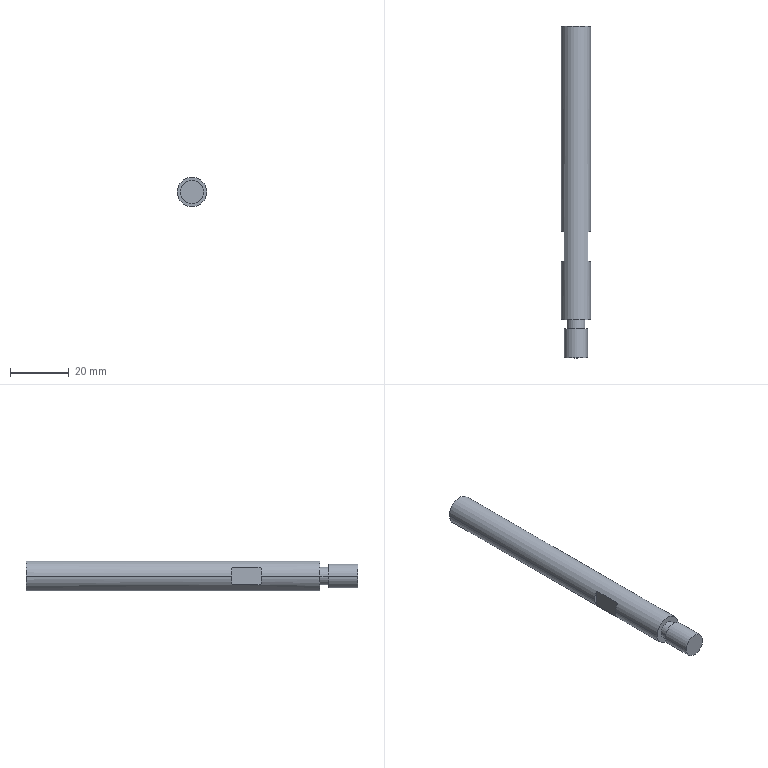Part | SolidWorks | features HoleWzd 1, ICE 1, Revolution 1 | 1 solid | 20 faces | box 10 x 113 x 10 mm | volume 8114 mm3 | plane 10 | cylinder 8 | cone 2 | commonest cylinder face diameters 5 x2 6 x2 8 x2 10 x2
STEP:
#1=CARTESIAN_POINT('',(0.,2.171,-2.5));
#2=VERTEX_POINT('',#1);
#3=CARTESIAN_POINT('',(0.,2.171,2.5));
#4=VERTEX_POINT('',#3);
#5=CARTESIAN_POINT('',(0.,2.171,0.));
#6=DIRECTION('',(0.,1.,0.));
#7=DIRECTION('',(0.,0.,1.));
#8=AXIS2_PLACEMENT_3D('',#5,#6,#7);
#9=CIRCLE('',#8,2.5);
#10=EDGE_CURVE('',#2,#4,#9,.T.);
#11=ORIENTED_EDGE('',*,*,#10,.F.);
#12=CARTESIAN_POINT('',(0.,14.171,-2.5));
#13=VERTEX_POINT('',#12);
#14=CARTESIAN_POINT('',(0.,14.171,-2.5));
#15=DIRECTION('',(0.,1.,0.));
#16=VECTOR('',#15,1000.);
#17=LINE('',#14,#16);
#18=EDGE_CURVE('',#2,#13,#17,.T.);
#19=ORIENTED_EDGE('',*,*,#18,.T.);
#20=CARTESIAN_POINT('',(0.,14.171,2.5));
#21=VERTEX_POINT('',#20);
#22=CARTESIAN_POINT('',(0.,14.171,0.));
#23=DIRECTION('',(0.,1.,0.));
#24=DIRECTION('',(0.,0.,1.));
#25=AXIS2_PLACEMENT_3D('',#22,#23,#24);
#26=CIRCLE('',#25,2.5);
#27=EDGE_CURVE('',#13,#21,#26,.T.);
#28=ORIENTED_EDGE('',*,*,#27,.T.);
#29=CARTESIAN_POINT('',(0.,14.171,2.5));
#30=DIRECTION('',(0.,1.,0.));
#31=VECTOR('',#30,1000.);
#32=LINE('',#29,#31);
#33=EDGE_CURVE('',#4,#21,#32,.T.);
#34=ORIENTED_EDGE('',*,*,#33,.F.);
#35=EDGE_LOOP('',(#11,#19,#28,#34));
#36=FACE_OUTER_BOUND('',#35,.T.);
#37=CARTESIAN_POINT('',(0.,14.171,0.));
#38=DIRECTION('',(0.,1.,0.));
#39=DIRECTION('',(0.,0.,1.));
#40=AXIS2_PLACEMENT_3D('',#37,#38,#39);
#41=CYLINDRICAL_SURFACE('',#40,2.5);
#42=ADVANCED_FACE('',(#36),#41,.F.);
#43=CARTESIAN_POINT('',(0.,0.6688,0.));
#44=VERTEX_POINT('',#43);
#45=CARTESIAN_POINT('',(0.,2.171,2.5));
#46=DIRECTION('',(0.,0.515,0.8572));
#47=VECTOR('',#46,1000.);
#48=LINE('',#45,#47);
#49=EDGE_CURVE('',#44,#4,#48,.T.);
#50=ORIENTED_EDGE('',*,*,#49,.F.);
#51=CARTESIAN_POINT('',(0.,2.171,-2.5));
#52=DIRECTION('',(0.,0.515,-0.8572));
#53=VECTOR('',#52,1000.);
#54=LINE('',#51,#53);
#55=EDGE_CURVE('',#44,#2,#54,.T.);
#56=ORIENTED_EDGE('',*,*,#55,.T.);
#57=ORIENTED_EDGE('',*,*,#10,.T.);
#58=EDGE_LOOP('',(#50,#56,#57));
#59=FACE_OUTER_BOUND('',#58,.T.);
#60=CARTESIAN_POINT('',(0.,2.171,0.));
#61=DIRECTION('',(0.,1.,0.));
#62=DIRECTION('',(0.,0.,1.));
#63=AXIS2_PLACEMENT_3D('',#60,#61,#62);
#64=CONICAL_SURFACE('',#63,2.5,1.03);
#65=ADVANCED_FACE('',(#59),#64,.F.);
#66=CARTESIAN_POINT('',(-5.,-85.829,0.));
#67=VERTEX_POINT('',#66);
#68=CARTESIAN_POINT('',(5.,-85.829,0.));
#69=VERTEX_POINT('',#68);
#70=CARTESIAN_POINT('',(0.,-85.829,0.));
#71=DIRECTION('',(0.,1.,0.));
#72=DIRECTION('',(-1.,0.,0.));
#73=AXIS2_PLACEMENT_3D('',#70,#71,#72);
#74=CIRCLE('',#73,5.);
#75=EDGE_CURVE('',#67,#69,#74,.T.);
#76=ORIENTED_EDGE('',*,*,#75,.T.);
#77=CARTESIAN_POINT('',(5.,-65.829,0.));
#78=VERTEX_POINT('',#77);
#79=CARTESIAN_POINT('',(5.,14.171,0.));
#80=DIRECTION('',(0.,1.,0.));
#81=VECTOR('',#80,1000.);
#82=LINE('',#79,#81);
#83=EDGE_CURVE('',#69,#78,#82,.T.);
#84=ORIENTED_EDGE('',*,*,#83,.T.);
#85=CARTESIAN_POINT('',(4.,-65.829,3.));
#86=VERTEX_POINT('',#85);
#87=CARTESIAN_POINT('',(0.,-65.829,0.));
#88=DIRECTION('',(0.,1.,0.));
#89=DIRECTION('',(0.,0.,-1.));
#90=AXIS2_PLACEMENT_3D('',#87,#88,#89);
#91=CIRCLE('',#90,5.);
#92=EDGE_CURVE('',#86,#78,#91,.T.);
#93=ORIENTED_EDGE('',*,*,#92,.F.);
#94=CARTESIAN_POINT('',(4.,-55.829,3.));
#95=VERTEX_POINT('',#94);
#96=CARTESIAN_POINT('',(4.,14.171,3.));
#97=DIRECTION('',(0.,-1.,0.));
#98=VECTOR('',#97,1000.);
#99=LINE('',#96,#98);
#100=EDGE_CURVE('',#95,#86,#99,.T.);
#101=ORIENTED_EDGE('',*,*,#100,.F.);
#102=CARTESIAN_POINT('',(5.,-55.829,0.));
#103=VERTEX_POINT('',#102);
#104=CARTESIAN_POINT('',(0.,-55.829,0.));
#105=DIRECTION('',(0.,-1.,0.));
#106=DIRECTION('',(0.,0.,1.));
#107=AXIS2_PLACEMENT_3D('',#104,#105,#106);
#108=CIRCLE('',#107,5.);
#109=EDGE_CURVE('',#103,#95,#108,.T.);
#110=ORIENTED_EDGE('',*,*,#109,.F.);
#111=CARTESIAN_POINT('',(5.,14.171,0.));
#112=VERTEX_POINT('',#111);
#113=CARTESIAN_POINT('',(5.,14.171,0.));
#114=DIRECTION('',(0.,1.,0.));
#115=VECTOR('',#114,1000.);
#116=LINE('',#113,#115);
#117=EDGE_CURVE('',#103,#112,#116,.T.);
#118=ORIENTED_EDGE('',*,*,#117,.T.);
#119=CARTESIAN_POINT('',(-5.,14.171,0.));
#120=VERTEX_POINT('',#119);
#121=CARTESIAN_POINT('',(0.,14.171,0.));
#122=DIRECTION('',(0.,1.,0.));
#123=DIRECTION('',(-1.,0.,0.));
#124=AXIS2_PLACEMENT_3D('',#121,#122,#123);
#125=CIRCLE('',#124,5.);
#126=EDGE_CURVE('',#120,#112,#125,.T.);
#127=ORIENTED_EDGE('',*,*,#126,.F.);
#128=CARTESIAN_POINT('',(-5.,-55.829,0.));
#129=VERTEX_POINT('',#128);
#130=CARTESIAN_POINT('',(-5.,14.171,0.));
#131=DIRECTION('',(0.,1.,0.));
#132=VECTOR('',#131,1000.);
#133=LINE('',#130,#132);
#134=EDGE_CURVE('',#129,#120,#133,.T.);
#135=ORIENTED_EDGE('',*,*,#134,.F.);
#136=CARTESIAN_POINT('',(-4.,-55.829,3.));
#137=VERTEX_POINT('',#136);
#138=CARTESIAN_POINT('',(0.,-55.829,0.));
#139=DIRECTION('',(0.,-1.,0.));
#140=DIRECTION('',(0.,0.,1.));
#141=AXIS2_PLACEMENT_3D('',#138,#139,#140);
#142=CIRCLE('',#141,5.);
#143=EDGE_CURVE('',#137,#129,#142,.T.);
#144=ORIENTED_EDGE('',*,*,#143,.F.);
#145=CARTESIAN_POINT('',(-4.,-65.829,3.));
#146=VERTEX_POINT('',#145);
#147=CARTESIAN_POINT('',(-4.,14.171,3.));
#148=DIRECTION('',(0.,1.,0.));
#149=VECTOR('',#148,1000.);
#150=LINE('',#147,#149);
#151=EDGE_CURVE('',#146,#137,#150,.T.);
#152=ORIENTED_EDGE('',*,*,#151,.F.);
#153=CARTESIAN_POINT('',(-5.,-65.829,0.));
#154=VERTEX_POINT('',#153);
#155=CARTESIAN_POINT('',(0.,-65.829,0.));
#156=DIRECTION('',(0.,1.,0.));
#157=DIRECTION('',(0.,0.,-1.));
#158=AXIS2_PLACEMENT_3D('',#155,#156,#157);
#159=CIRCLE('',#158,5.);
#160=EDGE_CURVE('',#154,#146,#159,.T.);
#161=ORIENTED_EDGE('',*,*,#160,.F.);
#162=CARTESIAN_POINT('',(-5.,14.171,0.));
#163=DIRECTION('',(0.,1.,0.));
#164=VECTOR('',#163,1000.);
#165=LINE('',#162,#164);
#166=EDGE_CURVE('',#67,#154,#165,.T.);
#167=ORIENTED_EDGE('',*,*,#166,.F.);
#168=EDGE_LOOP('',(#76,#84,#93,#101,#110,#118,#127,#135,#144,#152,#161,#167));
#169=FACE_OUTER_BOUND('',#168,.T.);
#170=CARTESIAN_POINT('',(0.,14.171,0.));
#171=DIRECTION('',(0.,1.,0.));
#172=DIRECTION('',(-1.,0.,0.));
#173=AXIS2_PLACEMENT_3D('',#170,#171,#172);
#174=CYLINDRICAL_SURFACE('',#173,5.);
#175=ADVANCED_FACE('',(#169),#174,.T.);
#176=CARTESIAN_POINT('',(-3.,-88.829,0.));
#177=VERTEX_POINT('',#176);
#178=CARTESIAN_POINT('',(3.,-88.829,0.));
#179=VERTEX_POINT('',#178);
#180=CARTESIAN_POINT('',(0.,-88.829,0.));
#181=DIRECTION('',(0.,1.,0.));
#182=DIRECTION('',(-1.,0.,0.));
#183=AXIS2_PLACEMENT_3D('',#180,#181,#182);
#184=CIRCLE('',#183,3.);
#185=EDGE_CURVE('',#177,#179,#184,.T.);
#186=ORIENTED_EDGE('',*,*,#185,.T.);
#187=CARTESIAN_POINT('',(3.,-85.829,0.));
#188=VERTEX_POINT('',#187);
#189=CARTESIAN_POINT('',(3.,14.171,0.));
#190=DIRECTION('',(0.,1.,0.));
#191=VECTOR('',#190,1000.);
#192=LINE('',#189,#191);
#193=EDGE_CURVE('',#179,#188,#192,.T.);
#194=ORIENTED_EDGE('',*,*,#193,.T.);
#195=CARTESIAN_POINT('',(-3.,-85.829,0.));
#196=VERTEX_POINT('',#195);
#197=CARTESIAN_POINT('',(0.,-85.829,0.));
#198=DIRECTION('',(0.,1.,0.));
#199=DIRECTION('',(-1.,0.,0.));
#200=AXIS2_PLACEMENT_3D('',#197,#198,#199);
#201=CIRCLE('',#200,3.);
#202=EDGE_CURVE('',#196,#188,#201,.T.);
#203=ORIENTED_EDGE('',*,*,#202,.F.);
#204=CARTESIAN_POINT('',(-3.,14.171,0.));
#205=DIRECTION('',(0.,1.,0.));
#206=VECTOR('',#205,1000.);
#207=LINE('',#204,#206);
#208=EDGE_CURVE('',#177,#196,#207,.T.);
#209=ORIENTED_EDGE('',*,*,#208,.F.);
#210=EDGE_LOOP('',(#186,#194,#203,#209));
#211=FACE_OUTER_BOUND('',#210,.T.);
#212=CARTESIAN_POINT('',(0.,14.171,0.));
#213=DIRECTION('',(0.,1.,0.));
#214=DIRECTION('',(-1.,0.,0.));
#215=AXIS2_PLACEMENT_3D('',#212,#213,#214);
#216=CYLINDRICAL_SURFACE('',#215,3.);
#217=ADVANCED_FACE('',(#211),#216,.T.);
#218=CARTESIAN_POINT('',(-4.,-98.829,0.));
#219=VERTEX_POINT('',#218);
#220=CARTESIAN_POINT('',(4.,-98.829,0.));
#221=VERTEX_POINT('',#220);
#222=CARTESIAN_POINT('',(0.,-98.829,0.));
#223=DIRECTION('',(0.,1.,0.));
#224=DIRECTION('',(-1.,0.,0.));
#225=AXIS2_PLACEMENT_3D('',#222,#223,#224);
#226=CIRCLE('',#225,4.);
#227=EDGE_CURVE('',#219,#221,#226,.T.);
#228=ORIENTED_EDGE('',*,*,#227,.T.);
#229=CARTESIAN_POINT('',(4.,-88.829,0.));
#230=VERTEX_POINT('',#229);
#231=CARTESIAN_POINT('',(4.,14.171,0.));
#232=DIRECTION('',(0.,1.,0.));
#233=VECTOR('',#232,1000.);
#234=LINE('',#231,#233);
#235=EDGE_CURVE('',#221,#230,#234,.T.);
#236=ORIENTED_EDGE('',*,*,#235,.T.);
#237=CARTESIAN_POINT('',(-4.,-88.829,0.));
#238=VERTEX_POINT('',#237);
#239=CARTESIAN_POINT('',(0.,-88.829,0.));
#240=DIRECTION('',(0.,1.,0.));
#241=DIRECTION('',(-1.,0.,0.));
#242=AXIS2_PLACEMENT_3D('',#239,#240,#241);
#243=CIRCLE('',#242,4.);
#244=EDGE_CURVE('',#238,#230,#243,.T.);
#245=ORIENTED_EDGE('',*,*,#244,.F.);
#246=CARTESIAN_POINT('',(-4.,14.171,0.));
#247=DIRECTION('',(0.,1.,0.));
#248=VECTOR('',#247,1000.);
#249=LINE('',#246,#248);
#250=EDGE_CURVE('',#219,#238,#249,.T.);
#251=ORIENTED_EDGE('',*,*,#250,.F.);
#252=EDGE_LOOP('',(#228,#236,#245,#251));
#253=FACE_OUTER_BOUND('',#252,.T.);
#254=CARTESIAN_POINT('',(0.,14.171,0.));
#255=DIRECTION('',(0.,1.,0.));
#256=DIRECTION('',(-1.,0.,0.));
#257=AXIS2_PLACEMENT_3D('',#254,#255,#256);
#258=CYLINDRICAL_SURFACE('',#257,4.);
#259=ADVANCED_FACE('',(#253),#258,.T.);
#260=CARTESIAN_POINT('',(0.,14.171,0.));
#261=DIRECTION('',(0.,1.,0.));
#262=DIRECTION('',(0.,0.,1.));
#263=AXIS2_PLACEMENT_3D('',#260,#261,#262);
#264=CIRCLE('',#263,2.5);
#265=EDGE_CURVE('',#21,#13,#264,.T.);
#266=ORIENTED_EDGE('',*,*,#265,.F.);
#267=ORIENTED_EDGE('',*,*,#27,.F.);
#268=EDGE_LOOP('',(#266,#267));
#269=FACE_BOUND('',#268,.T.);
#270=ORIENTED_EDGE('',*,*,#126,.T.);
#271=CARTESIAN_POINT('',(0.,14.171,0.));
#272=DIRECTION('',(0.,1.,0.));
#273=DIRECTION('',(-1.,0.,0.));
#274=AXIS2_PLACEMENT_3D('',#271,#272,#273);
#275=CIRCLE('',#274,5.);
#276=EDGE_CURVE('',#112,#120,#275,.T.);
#277=ORIENTED_EDGE('',*,*,#276,.T.);
#278=EDGE_LOOP('',(#270,#277));
#279=FACE_OUTER_BOUND('',#278,.T.);
#280=CARTESIAN_POINT('',(-5.,14.171,0.));
#281=DIRECTION('',(0.,1.,0.));
#282=DIRECTION('',(-1.,0.,0.));
#283=AXIS2_PLACEMENT_3D('',#280,#281,#282);
#284=PLANE('',#283);
#285=ADVANCED_FACE('',(#269,#279),#284,.T.);
#286=ORIENTED_EDGE('',*,*,#227,.F.);
#287=CARTESIAN_POINT('',(0.,-98.829,0.));
#288=DIRECTION('',(0.,1.,0.));
#289=DIRECTION('',(-1.,0.,0.));
#290=AXIS2_PLACEMENT_3D('',#287,#288,#289);
#291=CIRCLE('',#290,4.);
#292=EDGE_CURVE('',#221,#219,#291,.T.);
#293=ORIENTED_EDGE('',*,*,#292,.F.);
#294=EDGE_LOOP('',(#286,#293));
#295=FACE_OUTER_BOUND('',#294,.T.);
#296=CARTESIAN_POINT('',(0.,-98.829,0.));
#297=DIRECTION('',(0.,-1.,0.));
#298=DIRECTION('',(1.,0.,0.));
#299=AXIS2_PLACEMENT_3D('',#296,#297,#298);
#300=PLANE('',#299);
#301=ADVANCED_FACE('',(#295),#300,.T.);
#302=ORIENTED_EDGE('',*,*,#235,.F.);
#303=ORIENTED_EDGE('',*,*,#292,.T.);
#304=ORIENTED_EDGE('',*,*,#250,.T.);
#305=CARTESIAN_POINT('',(0.,-88.829,0.));
#306=DIRECTION('',(0.,1.,0.));
#307=DIRECTION('',(-1.,0.,0.));
#308=AXIS2_PLACEMENT_3D('',#305,#306,#307);
#309=CIRCLE('',#308,4.);
#310=EDGE_CURVE('',#230,#238,#309,.T.);
#311=ORIENTED_EDGE('',*,*,#310,.F.);
#312=EDGE_LOOP('',(#302,#303,#304,#311));
#313=FACE_OUTER_BOUND('',#312,.T.);
#314=CARTESIAN_POINT('',(0.,14.171,0.));
#315=DIRECTION('',(0.,1.,0.));
#316=DIRECTION('',(-1.,0.,0.));
#317=AXIS2_PLACEMENT_3D('',#314,#315,#316);
#318=CYLINDRICAL_SURFACE('',#317,4.);
#319=ADVANCED_FACE('',(#313),#318,.T.);
#320=ORIENTED_EDGE('',*,*,#244,.T.);
#321=ORIENTED_EDGE('',*,*,#310,.T.);
#322=EDGE_LOOP('',(#320,#321));
#323=FACE_OUTER_BOUND('',#322,.T.);
#324=ORIENTED_EDGE('',*,*,#185,.F.);
#325=CARTESIAN_POINT('',(0.,-88.829,0.));
#326=DIRECTION('',(0.,1.,0.));
#327=DIRECTION('',(-1.,0.,0.));
#328=AXIS2_PLACEMENT_3D('',#325,#326,#327);
#329=CIRCLE('',#328,3.);
#330=EDGE_CURVE('',#179,#177,#329,.T.);
#331=ORIENTED_EDGE('',*,*,#330,.F.);
#332=EDGE_LOOP('',(#324,#331));
#333=FACE_BOUND('',#332,.T.);
#334=CARTESIAN_POINT('',(-4.,-88.829,0.));
#335=DIRECTION('',(0.,1.,0.));
#336=DIRECTION('',(-1.,0.,0.));
#337=AXIS2_PLACEMENT_3D('',#334,#335,#336);
#338=PLANE('',#337);
#339=ADVANCED_FACE('',(#323,#333),#338,.T.);
#340=ORIENTED_EDGE('',*,*,#193,.F.);
#341=ORIENTED_EDGE('',*,*,#330,.T.);
#342=ORIENTED_EDGE('',*,*,#208,.T.);
#343=CARTESIAN_POINT('',(0.,-85.829,0.));
#344=DIRECTION('',(0.,1.,0.));
#345=DIRECTION('',(-1.,0.,0.));
#346=AXIS2_PLACEMENT_3D('',#343,#344,#345);
#347=CIRCLE('',#346,3.);
#348=EDGE_CURVE('',#188,#196,#347,.T.);
#349=ORIENTED_EDGE('',*,*,#348,.F.);
#350=EDGE_LOOP('',(#340,#341,#342,#349));
#351=FACE_OUTER_BOUND('',#350,.T.);
#352=CARTESIAN_POINT('',(0.,14.171,0.));
#353=DIRECTION('',(0.,1.,0.));
#354=DIRECTION('',(-1.,0.,0.));
#355=AXIS2_PLACEMENT_3D('',#352,#353,#354);
#356=CYLINDRICAL_SURFACE('',#355,3.);
#357=ADVANCED_FACE('',(#351),#356,.T.);
#358=ORIENTED_EDGE('',*,*,#202,.T.);
#359=ORIENTED_EDGE('',*,*,#348,.T.);
#360=EDGE_LOOP('',(#358,#359));
#361=FACE_BOUND('',#360,.T.);
#362=ORIENTED_EDGE('',*,*,#75,.F.);
#363=CARTESIAN_POINT('',(0.,-85.829,0.));
#364=DIRECTION('',(0.,1.,0.));
#365=DIRECTION('',(-1.,0.,0.));
#366=AXIS2_PLACEMENT_3D('',#363,#364,#365);
#367=CIRCLE('',#366,5.);
#368=EDGE_CURVE('',#69,#67,#367,.T.);
#369=ORIENTED_EDGE('',*,*,#368,.F.);
#370=EDGE_LOOP('',(#362,#369));
#371=FACE_OUTER_BOUND('',#370,.T.);
#372=CARTESIAN_POINT('',(-3.,-85.829,0.));
#373=DIRECTION('',(0.,-1.,0.));
#374=DIRECTION('',(1.,0.,0.));
#375=AXIS2_PLACEMENT_3D('',#372,#373,#374);
#376=PLANE('',#375);
#377=ADVANCED_FACE('',(#361,#371),#376,.T.);
#378=ORIENTED_EDGE('',*,*,#83,.F.);
#379=ORIENTED_EDGE('',*,*,#368,.T.);
#380=ORIENTED_EDGE('',*,*,#166,.T.);
#381=CARTESIAN_POINT('',(-4.,-65.829,-3.));
#382=VERTEX_POINT('',#381);
#383=CARTESIAN_POINT('',(0.,-65.829,0.));
#384=DIRECTION('',(0.,1.,0.));
#385=DIRECTION('',(0.,0.,-1.));
#386=AXIS2_PLACEMENT_3D('',#383,#384,#385);
#387=CIRCLE('',#386,5.);
#388=EDGE_CURVE('',#382,#154,#387,.T.);
#389=ORIENTED_EDGE('',*,*,#388,.F.);
#390=CARTESIAN_POINT('',(-4.,-55.829,-3.));
#391=VERTEX_POINT('',#390);
#392=CARTESIAN_POINT('',(-4.,14.171,-3.));
#393=DIRECTION('',(0.,-1.,0.));
#394=VECTOR('',#393,1000.);
#395=LINE('',#392,#394);
#396=EDGE_CURVE('',#391,#382,#395,.T.);
#397=ORIENTED_EDGE('',*,*,#396,.F.);
#398=CARTESIAN_POINT('',(0.,-55.829,0.));
#399=DIRECTION('',(0.,-1.,0.));
#400=DIRECTION('',(0.,0.,1.));
#401=AXIS2_PLACEMENT_3D('',#398,#399,#400);
#402=CIRCLE('',#401,5.);
#403=EDGE_CURVE('',#129,#391,#402,.T.);
#404=ORIENTED_EDGE('',*,*,#403,.F.);
#405=ORIENTED_EDGE('',*,*,#134,.T.);
#406=ORIENTED_EDGE('',*,*,#276,.F.);
#407=ORIENTED_EDGE('',*,*,#117,.F.);
#408=CARTESIAN_POINT('',(4.,-55.829,-3.));
#409=VERTEX_POINT('',#408);
#410=CARTESIAN_POINT('',(0.,-55.829,0.));
#411=DIRECTION('',(0.,-1.,0.));
#412=DIRECTION('',(0.,0.,1.));
#413=AXIS2_PLACEMENT_3D('',#410,#411,#412);
#414=CIRCLE('',#413,5.);
#415=EDGE_CURVE('',#409,#103,#414,.T.);
#416=ORIENTED_EDGE('',*,*,#415,.F.);
#417=CARTESIAN_POINT('',(4.,-65.829,-3.));
#418=VERTEX_POINT('',#417);
#419=CARTESIAN_POINT('',(4.,14.171,-3.));
#420=DIRECTION('',(0.,1.,0.));
#421=VECTOR('',#420,1000.);
#422=LINE('',#419,#421);
#423=EDGE_CURVE('',#418,#409,#422,.T.);
#424=ORIENTED_EDGE('',*,*,#423,.F.);
#425=CARTESIAN_POINT('',(0.,-65.829,0.));
#426=DIRECTION('',(0.,1.,0.));
#427=DIRECTION('',(0.,0.,-1.));
#428=AXIS2_PLACEMENT_3D('',#425,#426,#427);
#429=CIRCLE('',#428,5.);
#430=EDGE_CURVE('',#78,#418,#429,.T.);
#431=ORIENTED_EDGE('',*,*,#430,.F.);
#432=EDGE_LOOP('',(#378,#379,#380,#389,#397,#404,#405,#406,#407,#416,#424,#431));
#433=FACE_OUTER_BOUND('',#432,.T.);
#434=CARTESIAN_POINT('',(0.,14.171,0.));
#435=DIRECTION('',(0.,1.,0.));
#436=DIRECTION('',(-1.,0.,0.));
#437=AXIS2_PLACEMENT_3D('',#434,#435,#436);
#438=CYLINDRICAL_SURFACE('',#437,5.);
#439=ADVANCED_FACE('',(#433),#438,.T.);
#440=ORIENTED_EDGE('',*,*,#415,.T.);
#441=ORIENTED_EDGE('',*,*,#109,.T.);
#442=CARTESIAN_POINT('',(4.,-55.829,-5.));
#443=DIRECTION('',(0.,0.,1.));
#444=VECTOR('',#443,1000.);
#445=LINE('',#442,#444);
#446=EDGE_CURVE('',#409,#95,#445,.T.);
#447=ORIENTED_EDGE('',*,*,#446,.F.);
#448=EDGE_LOOP('',(#440,#441,#447));
#449=FACE_OUTER_BOUND('',#448,.T.);
#450=CARTESIAN_POINT('',(5.,-55.829,-5.));
#451=DIRECTION('',(0.,1.,0.));
#452=DIRECTION('',(0.,0.,1.));
#453=AXIS2_PLACEMENT_3D('',#450,#451,#452);
#454=PLANE('',#453);
#455=ADVANCED_FACE('',(#449),#454,.F.);
#456=CARTESIAN_POINT('',(4.,-65.829,-5.));
#457=DIRECTION('',(0.,0.,1.));
#458=VECTOR('',#457,1000.);
#459=LINE('',#456,#458);
#460=EDGE_CURVE('',#418,#86,#459,.T.);
#461=ORIENTED_EDGE('',*,*,#460,.T.);
#462=ORIENTED_EDGE('',*,*,#92,.T.);
#463=ORIENTED_EDGE('',*,*,#430,.T.);
#464=EDGE_LOOP('',(#461,#462,#463));
#465=FACE_OUTER_BOUND('',#464,.T.);
#466=CARTESIAN_POINT('',(5.,-65.829,-5.));
#467=DIRECTION('',(0.,-1.,0.));
#468=DIRECTION('',(0.,0.,-1.));
#469=AXIS2_PLACEMENT_3D('',#466,#467,#468);
#470=PLANE('',#469);
#471=ADVANCED_FACE('',(#465),#470,.F.);
#472=ORIENTED_EDGE('',*,*,#100,.T.);
#473=ORIENTED_EDGE('',*,*,#460,.F.);
#474=ORIENTED_EDGE('',*,*,#423,.T.);
#475=ORIENTED_EDGE('',*,*,#446,.T.);
#476=EDGE_LOOP('',(#472,#473,#474,#475));
#477=FACE_OUTER_BOUND('',#476,.T.);
#478=CARTESIAN_POINT('',(4.,-55.829,-5.));
#479=DIRECTION('',(-1.,0.,0.));
#480=DIRECTION('',(0.,-1.,0.));
#481=AXIS2_PLACEMENT_3D('',#478,#479,#480);
#482=PLANE('',#481);
#483=ADVANCED_FACE('',(#477),#482,.F.);
#484=CARTESIAN_POINT('',(-4.,-55.829,-5.));
#485=DIRECTION('',(0.,0.,1.));
#486=VECTOR('',#485,1000.);
#487=LINE('',#484,#486);
#488=EDGE_CURVE('',#391,#137,#487,.T.);
#489=ORIENTED_EDGE('',*,*,#488,.T.);
#490=ORIENTED_EDGE('',*,*,#143,.T.);
#491=ORIENTED_EDGE('',*,*,#403,.T.);
#492=EDGE_LOOP('',(#489,#490,#491));
#493=FACE_OUTER_BOUND('',#492,.T.);
#494=CARTESIAN_POINT('',(-5.,-55.829,-5.));
#495=DIRECTION('',(0.,1.,0.));
#496=DIRECTION('',(0.,0.,1.));
#497=AXIS2_PLACEMENT_3D('',#494,#495,#496);
#498=PLANE('',#497);
#499=ADVANCED_FACE('',(#493),#498,.F.);
#500=ORIENTED_EDGE('',*,*,#396,.T.);
#501=CARTESIAN_POINT('',(-4.,-65.829,-5.));
#502=DIRECTION('',(0.,0.,1.));
#503=VECTOR('',#502,1000.);
#504=LINE('',#501,#503);
#505=EDGE_CURVE('',#382,#146,#504,.T.);
#506=ORIENTED_EDGE('',*,*,#505,.T.);
#507=ORIENTED_EDGE('',*,*,#151,.T.);
#508=ORIENTED_EDGE('',*,*,#488,.F.);
#509=EDGE_LOOP('',(#500,#506,#507,#508));
#510=FACE_OUTER_BOUND('',#509,.T.);
#511=CARTESIAN_POINT('',(-4.,-55.829,-5.));
#512=DIRECTION('',(1.,0.,0.));
#513=DIRECTION('',(0.,1.,0.));
#514=AXIS2_PLACEMENT_3D('',#511,#512,#513);
#515=PLANE('',#514);
#516=ADVANCED_FACE('',(#510),#515,.F.);
#517=ORIENTED_EDGE('',*,*,#505,.F.);
#518=ORIENTED_EDGE('',*,*,#388,.T.);
#519=ORIENTED_EDGE('',*,*,#160,.T.);
#520=EDGE_LOOP('',(#517,#518,#519));
#521=FACE_OUTER_BOUND('',#520,.T.);
#522=CARTESIAN_POINT('',(-5.,-65.829,-5.));
#523=DIRECTION('',(0.,-1.,0.));
#524=DIRECTION('',(0.,0.,-1.));
#525=AXIS2_PLACEMENT_3D('',#522,#523,#524);
#526=PLANE('',#525);
#527=ADVANCED_FACE('',(#521),#526,.F.);
#528=ORIENTED_EDGE('',*,*,#55,.F.);
#529=ORIENTED_EDGE('',*,*,#49,.T.);
#530=CARTESIAN_POINT('',(0.,2.171,0.));
#531=DIRECTION('',(0.,1.,0.));
#532=DIRECTION('',(0.,0.,1.));
#533=AXIS2_PLACEMENT_3D('',#530,#531,#532);
#534=CIRCLE('',#533,2.5);
#535=EDGE_CURVE('',#4,#2,#534,.T.);
#536=ORIENTED_EDGE('',*,*,#535,.T.);
#537=EDGE_LOOP('',(#528,#529,#536));
#538=FACE_OUTER_BOUND('',#537,.T.);
#539=CARTESIAN_POINT('',(0.,2.171,0.));
#540=DIRECTION('',(0.,1.,0.));
#541=DIRECTION('',(0.,0.,1.));
#542=AXIS2_PLACEMENT_3D('',#539,#540,#541);
#543=CONICAL_SURFACE('',#542,2.5,1.03);
#544=ADVANCED_FACE('',(#538),#543,.F.);
#545=ORIENTED_EDGE('',*,*,#18,.F.);
#546=ORIENTED_EDGE('',*,*,#535,.F.);
#547=ORIENTED_EDGE('',*,*,#33,.T.);
#548=ORIENTED_EDGE('',*,*,#265,.T.);
#549=EDGE_LOOP('',(#545,#546,#547,#548));
#550=FACE_OUTER_BOUND('',#549,.T.);
#551=CARTESIAN_POINT('',(0.,14.171,0.));
#552=DIRECTION('',(0.,1.,0.));
#553=DIRECTION('',(0.,0.,1.));
#554=AXIS2_PLACEMENT_3D('',#551,#552,#553);
#555=CYLINDRICAL_SURFACE('',#554,2.5);
#556=ADVANCED_FACE('',(#550),#555,.F.);
#557=CLOSED_SHELL('',(#42,#65,#175,#217,#259,#285,#301,#319,#339,#357,#377,#439,#455,#471,#483,#499,#516,#527,#544,#556));
#558=MANIFOLD_SOLID_BREP('',#557);
#559=CARTESIAN_POINT('',(0.,0.,0.));
#560=DIRECTION('',(0.,0.,1.));
#561=DIRECTION('',(1.,0.,0.));
#562=AXIS2_PLACEMENT_3D('',#559,#560,#561);
#563=(LENGTH_UNIT()NAMED_UNIT(*)SI_UNIT(.MILLI.,.METRE.));
#564=UNCERTAINTY_MEASURE_WITH_UNIT(LENGTH_MEASURE(0.00001),#563,'','');
#565=(NAMED_UNIT(*)PLANE_ANGLE_UNIT()SI_UNIT($,.RADIAN.));
#566=(NAMED_UNIT(*)SI_UNIT($,.STERADIAN.)SOLID_ANGLE_UNIT());
#567=(GEOMETRIC_REPRESENTATION_CONTEXT(3)GLOBAL_UNCERTAINTY_ASSIGNED_CONTEXT((#564))GLOBAL_UNIT_ASSIGNED_CONTEXT((#563,#565,#566))REPRESENTATION_CONTEXT('',''));
#568=ADVANCED_BREP_SHAPE_REPRESENTATION('',(#558,#562),#567);